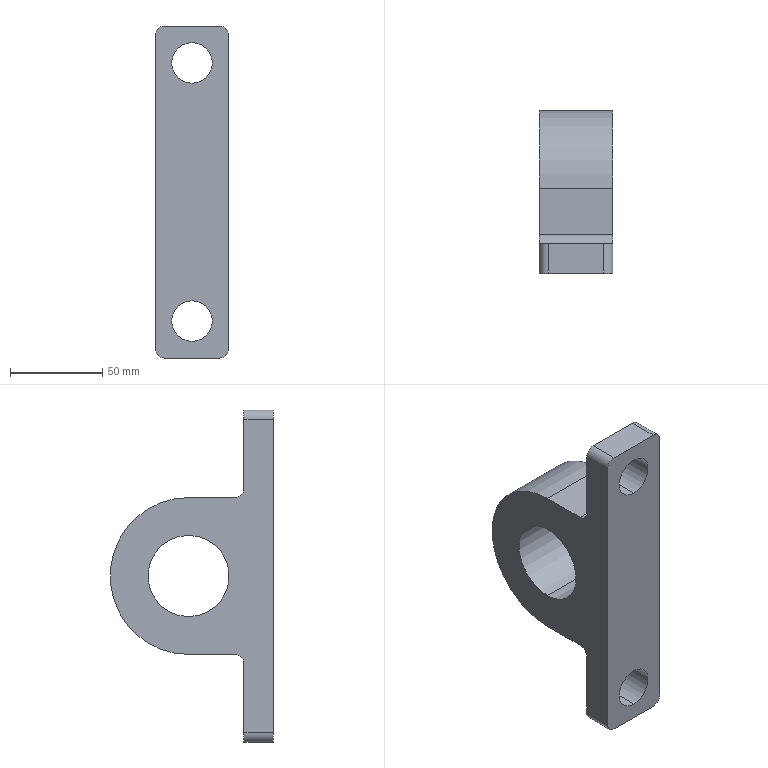Part | SolidWorks | features Extrusion 1, Fillet 1, ICE 1 | 1 solid | 22 faces | box 40 x 88.5 x 180 mm | volume 257790 mm3 | cylinder 13 | plane 9 | commonest cylinder face diameters 10 x6 22 x4 44 x2 85 x1
STEP:
#1=CARTESIAN_POINT('',(20.,46.,22.));
#2=VERTEX_POINT('',#1);
#3=CARTESIAN_POINT('',(20.,46.,-22.));
#4=VERTEX_POINT('',#3);
#5=CARTESIAN_POINT('',(20.,46.,0.));
#6=DIRECTION('',(1.,0.,0.));
#7=DIRECTION('',(0.,0.,-1.));
#8=AXIS2_PLACEMENT_3D('',#5,#6,#7);
#9=CIRCLE('',#8,22.);
#10=EDGE_CURVE('',#2,#4,#9,.T.);
#11=ORIENTED_EDGE('',*,*,#10,.T.);
#12=CARTESIAN_POINT('',(-20.,46.,-22.));
#13=VERTEX_POINT('',#12);
#14=CARTESIAN_POINT('',(20.,46.,-22.));
#15=DIRECTION('',(-1.,0.,0.));
#16=VECTOR('',#15,1000.);
#17=LINE('',#14,#16);
#18=EDGE_CURVE('',#4,#13,#17,.T.);
#19=ORIENTED_EDGE('',*,*,#18,.T.);
#20=CARTESIAN_POINT('',(-20.,46.,22.));
#21=VERTEX_POINT('',#20);
#22=CARTESIAN_POINT('',(-20.,46.,0.));
#23=DIRECTION('',(1.,0.,0.));
#24=DIRECTION('',(0.,0.,-1.));
#25=AXIS2_PLACEMENT_3D('',#22,#23,#24);
#26=CIRCLE('',#25,22.);
#27=EDGE_CURVE('',#21,#13,#26,.T.);
#28=ORIENTED_EDGE('',*,*,#27,.F.);
#29=CARTESIAN_POINT('',(20.,46.,22.));
#30=DIRECTION('',(-1.,0.,0.));
#31=VECTOR('',#30,1000.);
#32=LINE('',#29,#31);
#33=EDGE_CURVE('',#2,#21,#32,.T.);
#34=ORIENTED_EDGE('',*,*,#33,.F.);
#35=EDGE_LOOP('',(#11,#19,#28,#34));
#36=FACE_OUTER_BOUND('',#35,.T.);
#37=CARTESIAN_POINT('',(20.,46.,0.));
#38=DIRECTION('',(-1.,0.,0.));
#39=DIRECTION('',(0.,0.,1.));
#40=AXIS2_PLACEMENT_3D('',#37,#38,#39);
#41=CYLINDRICAL_SURFACE('',#40,22.);
#42=ADVANCED_FACE('',(#36),#41,.F.);
#43=CARTESIAN_POINT('',(0.,16.,59.));
#44=VERTEX_POINT('',#43);
#45=CARTESIAN_POINT('',(0.,16.,81.));
#46=VERTEX_POINT('',#45);
#47=CARTESIAN_POINT('',(0.,16.,70.));
#48=DIRECTION('',(0.,1.,0.));
#49=DIRECTION('',(0.,0.,-1.));
#50=AXIS2_PLACEMENT_3D('',#47,#48,#49);
#51=CIRCLE('',#50,11.);
#52=EDGE_CURVE('',#44,#46,#51,.T.);
#53=ORIENTED_EDGE('',*,*,#52,.T.);
#54=CARTESIAN_POINT('',(0.,0.,81.));
#55=VERTEX_POINT('',#54);
#56=CARTESIAN_POINT('',(0.,16.,81.));
#57=DIRECTION('',(0.,-1.,0.));
#58=VECTOR('',#57,1000.);
#59=LINE('',#56,#58);
#60=EDGE_CURVE('',#46,#55,#59,.T.);
#61=ORIENTED_EDGE('',*,*,#60,.T.);
#62=CARTESIAN_POINT('',(0.,0.,59.));
#63=VERTEX_POINT('',#62);
#64=CARTESIAN_POINT('',(0.,0.,70.));
#65=DIRECTION('',(0.,1.,0.));
#66=DIRECTION('',(0.,0.,-1.));
#67=AXIS2_PLACEMENT_3D('',#64,#65,#66);
#68=CIRCLE('',#67,11.);
#69=EDGE_CURVE('',#63,#55,#68,.T.);
#70=ORIENTED_EDGE('',*,*,#69,.F.);
#71=CARTESIAN_POINT('',(0.,16.,59.));
#72=DIRECTION('',(0.,-1.,0.));
#73=VECTOR('',#72,1000.);
#74=LINE('',#71,#73);
#75=EDGE_CURVE('',#44,#63,#74,.T.);
#76=ORIENTED_EDGE('',*,*,#75,.F.);
#77=EDGE_LOOP('',(#53,#61,#70,#76));
#78=FACE_OUTER_BOUND('',#77,.T.);
#79=CARTESIAN_POINT('',(0.,16.,70.));
#80=DIRECTION('',(0.,-1.,0.));
#81=DIRECTION('',(0.,0.,-1.));
#82=AXIS2_PLACEMENT_3D('',#79,#80,#81);
#83=CYLINDRICAL_SURFACE('',#82,11.);
#84=ADVANCED_FACE('',(#78),#83,.F.);
#85=CARTESIAN_POINT('',(0.,16.,-81.));
#86=VERTEX_POINT('',#85);
#87=CARTESIAN_POINT('',(0.,16.,-59.));
#88=VERTEX_POINT('',#87);
#89=CARTESIAN_POINT('',(0.,16.,-70.));
#90=DIRECTION('',(0.,1.,0.));
#91=DIRECTION('',(0.,0.,1.));
#92=AXIS2_PLACEMENT_3D('',#89,#90,#91);
#93=CIRCLE('',#92,11.);
#94=EDGE_CURVE('',#86,#88,#93,.T.);
#95=ORIENTED_EDGE('',*,*,#94,.T.);
#96=CARTESIAN_POINT('',(0.,0.,-59.));
#97=VERTEX_POINT('',#96);
#98=CARTESIAN_POINT('',(0.,16.,-59.));
#99=DIRECTION('',(0.,-1.,0.));
#100=VECTOR('',#99,1000.);
#101=LINE('',#98,#100);
#102=EDGE_CURVE('',#88,#97,#101,.T.);
#103=ORIENTED_EDGE('',*,*,#102,.T.);
#104=CARTESIAN_POINT('',(0.,0.,-81.));
#105=VERTEX_POINT('',#104);
#106=CARTESIAN_POINT('',(0.,0.,-70.));
#107=DIRECTION('',(0.,1.,0.));
#108=DIRECTION('',(0.,0.,1.));
#109=AXIS2_PLACEMENT_3D('',#106,#107,#108);
#110=CIRCLE('',#109,11.);
#111=EDGE_CURVE('',#105,#97,#110,.T.);
#112=ORIENTED_EDGE('',*,*,#111,.F.);
#113=CARTESIAN_POINT('',(0.,16.,-81.));
#114=DIRECTION('',(0.,-1.,0.));
#115=VECTOR('',#114,1000.);
#116=LINE('',#113,#115);
#117=EDGE_CURVE('',#86,#105,#116,.T.);
#118=ORIENTED_EDGE('',*,*,#117,.F.);
#119=EDGE_LOOP('',(#95,#103,#112,#118));
#120=FACE_OUTER_BOUND('',#119,.T.);
#121=CARTESIAN_POINT('',(0.,16.,-70.));
#122=DIRECTION('',(0.,-1.,0.));
#123=DIRECTION('',(0.,0.,-1.));
#124=AXIS2_PLACEMENT_3D('',#121,#122,#123);
#125=CYLINDRICAL_SURFACE('',#124,11.);
#126=ADVANCED_FACE('',(#120),#125,.F.);
#127=ORIENTED_EDGE('',*,*,#52,.F.);
#128=CARTESIAN_POINT('',(0.,16.,70.));
#129=DIRECTION('',(0.,1.,0.));
#130=DIRECTION('',(0.,0.,-1.));
#131=AXIS2_PLACEMENT_3D('',#128,#129,#130);
#132=CIRCLE('',#131,11.);
#133=EDGE_CURVE('',#46,#44,#132,.T.);
#134=ORIENTED_EDGE('',*,*,#133,.F.);
#135=EDGE_LOOP('',(#127,#134));
#136=FACE_BOUND('',#135,.T.);
#137=CARTESIAN_POINT('',(20.,16.,85.));
#138=VERTEX_POINT('',#137);
#139=CARTESIAN_POINT('',(20.,16.,47.5));
#140=VERTEX_POINT('',#139);
#141=CARTESIAN_POINT('',(20.,16.,-90.));
#142=DIRECTION('',(0.,0.,-1.));
#143=VECTOR('',#142,1000.);
#144=LINE('',#141,#143);
#145=EDGE_CURVE('',#138,#140,#144,.T.);
#146=ORIENTED_EDGE('',*,*,#145,.T.);
#147=CARTESIAN_POINT('',(-20.,16.,47.5));
#148=VERTEX_POINT('',#147);
#149=CARTESIAN_POINT('',(-20.,16.,47.5));
#150=DIRECTION('',(-1.,0.,0.));
#151=VECTOR('',#150,1000.);
#152=LINE('',#149,#151);
#153=EDGE_CURVE('',#140,#148,#152,.T.);
#154=ORIENTED_EDGE('',*,*,#153,.T.);
#155=CARTESIAN_POINT('',(-20.,16.,85.));
#156=VERTEX_POINT('',#155);
#157=CARTESIAN_POINT('',(-20.,16.,-90.));
#158=DIRECTION('',(0.,0.,1.));
#159=VECTOR('',#158,1000.);
#160=LINE('',#157,#159);
#161=EDGE_CURVE('',#148,#156,#160,.T.);
#162=ORIENTED_EDGE('',*,*,#161,.T.);
#163=CARTESIAN_POINT('',(-15.,16.,90.));
#164=VERTEX_POINT('',#163);
#165=CARTESIAN_POINT('',(-15.,16.,85.));
#166=DIRECTION('',(0.,1.,0.));
#167=DIRECTION('',(0.,0.,1.));
#168=AXIS2_PLACEMENT_3D('',#165,#166,#167);
#169=CIRCLE('',#168,5.);
#170=EDGE_CURVE('',#156,#164,#169,.T.);
#171=ORIENTED_EDGE('',*,*,#170,.T.);
#172=CARTESIAN_POINT('',(15.,16.,90.));
#173=VERTEX_POINT('',#172);
#174=CARTESIAN_POINT('',(-20.,16.,90.));
#175=DIRECTION('',(1.,0.,0.));
#176=VECTOR('',#175,1000.);
#177=LINE('',#174,#176);
#178=EDGE_CURVE('',#164,#173,#177,.T.);
#179=ORIENTED_EDGE('',*,*,#178,.T.);
#180=CARTESIAN_POINT('',(15.,16.,85.));
#181=DIRECTION('',(0.,1.,0.));
#182=DIRECTION('',(0.,0.,1.));
#183=AXIS2_PLACEMENT_3D('',#180,#181,#182);
#184=CIRCLE('',#183,5.);
#185=EDGE_CURVE('',#173,#138,#184,.T.);
#186=ORIENTED_EDGE('',*,*,#185,.T.);
#187=EDGE_LOOP('',(#146,#154,#162,#171,#179,#186));
#188=FACE_OUTER_BOUND('',#187,.T.);
#189=CARTESIAN_POINT('',(-20.,16.,90.));
#190=DIRECTION('',(0.,1.,0.));
#191=DIRECTION('',(0.,0.,1.));
#192=AXIS2_PLACEMENT_3D('',#189,#190,#191);
#193=PLANE('',#192);
#194=ADVANCED_FACE('',(#136,#188),#193,.T.);
#195=CARTESIAN_POINT('',(20.,16.,-47.5));
#196=VERTEX_POINT('',#195);
#197=CARTESIAN_POINT('',(20.,16.,-85.));
#198=VERTEX_POINT('',#197);
#199=CARTESIAN_POINT('',(20.,16.,-90.));
#200=DIRECTION('',(0.,0.,-1.));
#201=VECTOR('',#200,1000.);
#202=LINE('',#199,#201);
#203=EDGE_CURVE('',#196,#198,#202,.T.);
#204=ORIENTED_EDGE('',*,*,#203,.T.);
#205=CARTESIAN_POINT('',(15.,16.,-90.));
#206=VERTEX_POINT('',#205);
#207=CARTESIAN_POINT('',(15.,16.,-85.));
#208=DIRECTION('',(0.,1.,0.));
#209=DIRECTION('',(0.,0.,1.));
#210=AXIS2_PLACEMENT_3D('',#207,#208,#209);
#211=CIRCLE('',#210,5.);
#212=EDGE_CURVE('',#198,#206,#211,.T.);
#213=ORIENTED_EDGE('',*,*,#212,.T.);
#214=CARTESIAN_POINT('',(-15.,16.,-90.));
#215=VERTEX_POINT('',#214);
#216=CARTESIAN_POINT('',(-20.,16.,-90.));
#217=DIRECTION('',(-1.,0.,0.));
#218=VECTOR('',#217,1000.);
#219=LINE('',#216,#218);
#220=EDGE_CURVE('',#206,#215,#219,.T.);
#221=ORIENTED_EDGE('',*,*,#220,.T.);
#222=CARTESIAN_POINT('',(-20.,16.,-85.));
#223=VERTEX_POINT('',#222);
#224=CARTESIAN_POINT('',(-15.,16.,-85.));
#225=DIRECTION('',(0.,1.,0.));
#226=DIRECTION('',(0.,0.,1.));
#227=AXIS2_PLACEMENT_3D('',#224,#225,#226);
#228=CIRCLE('',#227,5.);
#229=EDGE_CURVE('',#215,#223,#228,.T.);
#230=ORIENTED_EDGE('',*,*,#229,.T.);
#231=CARTESIAN_POINT('',(-20.,16.,-47.5));
#232=VERTEX_POINT('',#231);
#233=CARTESIAN_POINT('',(-20.,16.,-90.));
#234=DIRECTION('',(0.,0.,1.));
#235=VECTOR('',#234,1000.);
#236=LINE('',#233,#235);
#237=EDGE_CURVE('',#223,#232,#236,.T.);
#238=ORIENTED_EDGE('',*,*,#237,.T.);
#239=CARTESIAN_POINT('',(-20.,16.,-47.5));
#240=DIRECTION('',(1.,0.,0.));
#241=VECTOR('',#240,1000.);
#242=LINE('',#239,#241);
#243=EDGE_CURVE('',#232,#196,#242,.T.);
#244=ORIENTED_EDGE('',*,*,#243,.T.);
#245=EDGE_LOOP('',(#204,#213,#221,#230,#238,#244));
#246=FACE_OUTER_BOUND('',#245,.T.);
#247=ORIENTED_EDGE('',*,*,#94,.F.);
#248=CARTESIAN_POINT('',(0.,16.,-70.));
#249=DIRECTION('',(0.,1.,0.));
#250=DIRECTION('',(0.,0.,1.));
#251=AXIS2_PLACEMENT_3D('',#248,#249,#250);
#252=CIRCLE('',#251,11.);
#253=EDGE_CURVE('',#88,#86,#252,.T.);
#254=ORIENTED_EDGE('',*,*,#253,.F.);
#255=EDGE_LOOP('',(#247,#254));
#256=FACE_BOUND('',#255,.T.);
#257=CARTESIAN_POINT('',(-20.,16.,90.));
#258=DIRECTION('',(0.,1.,0.));
#259=DIRECTION('',(0.,0.,1.));
#260=AXIS2_PLACEMENT_3D('',#257,#258,#259);
#261=PLANE('',#260);
#262=ADVANCED_FACE('',(#246,#256),#261,.T.);
#263=ORIENTED_EDGE('',*,*,#111,.T.);
#264=CARTESIAN_POINT('',(0.,0.,-70.));
#265=DIRECTION('',(0.,1.,0.));
#266=DIRECTION('',(0.,0.,1.));
#267=AXIS2_PLACEMENT_3D('',#264,#265,#266);
#268=CIRCLE('',#267,11.);
#269=EDGE_CURVE('',#97,#105,#268,.T.);
#270=ORIENTED_EDGE('',*,*,#269,.T.);
#271=EDGE_LOOP('',(#263,#270));
#272=FACE_BOUND('',#271,.T.);
#273=CARTESIAN_POINT('',(20.,0.,85.));
#274=VERTEX_POINT('',#273);
#275=CARTESIAN_POINT('',(20.,0.,-85.));
#276=VERTEX_POINT('',#275);
#277=CARTESIAN_POINT('',(20.,0.,-90.));
#278=DIRECTION('',(0.,0.,-1.));
#279=VECTOR('',#278,1000.);
#280=LINE('',#277,#279);
#281=EDGE_CURVE('',#274,#276,#280,.T.);
#282=ORIENTED_EDGE('',*,*,#281,.F.);
#283=CARTESIAN_POINT('',(15.,0.,90.));
#284=VERTEX_POINT('',#283);
#285=CARTESIAN_POINT('',(15.,0.,85.));
#286=DIRECTION('',(0.,-1.,0.));
#287=DIRECTION('',(0.,0.,1.));
#288=AXIS2_PLACEMENT_3D('',#285,#286,#287);
#289=CIRCLE('',#288,5.);
#290=EDGE_CURVE('',#274,#284,#289,.T.);
#291=ORIENTED_EDGE('',*,*,#290,.T.);
#292=CARTESIAN_POINT('',(-15.,0.,90.));
#293=VERTEX_POINT('',#292);
#294=CARTESIAN_POINT('',(-20.,0.,90.));
#295=DIRECTION('',(1.,0.,0.));
#296=VECTOR('',#295,1000.);
#297=LINE('',#294,#296);
#298=EDGE_CURVE('',#293,#284,#297,.T.);
#299=ORIENTED_EDGE('',*,*,#298,.F.);
#300=CARTESIAN_POINT('',(-20.,0.,85.));
#301=VERTEX_POINT('',#300);
#302=CARTESIAN_POINT('',(-15.,0.,85.));
#303=DIRECTION('',(0.,-1.,0.));
#304=DIRECTION('',(0.,0.,1.));
#305=AXIS2_PLACEMENT_3D('',#302,#303,#304);
#306=CIRCLE('',#305,5.);
#307=EDGE_CURVE('',#293,#301,#306,.T.);
#308=ORIENTED_EDGE('',*,*,#307,.T.);
#309=CARTESIAN_POINT('',(-20.,0.,-85.));
#310=VERTEX_POINT('',#309);
#311=CARTESIAN_POINT('',(-20.,0.,-90.));
#312=DIRECTION('',(0.,0.,1.));
#313=VECTOR('',#312,1000.);
#314=LINE('',#311,#313);
#315=EDGE_CURVE('',#310,#301,#314,.T.);
#316=ORIENTED_EDGE('',*,*,#315,.F.);
#317=CARTESIAN_POINT('',(-15.,0.,-90.));
#318=VERTEX_POINT('',#317);
#319=CARTESIAN_POINT('',(-15.,0.,-85.));
#320=DIRECTION('',(0.,-1.,0.));
#321=DIRECTION('',(0.,0.,1.));
#322=AXIS2_PLACEMENT_3D('',#319,#320,#321);
#323=CIRCLE('',#322,5.);
#324=EDGE_CURVE('',#310,#318,#323,.T.);
#325=ORIENTED_EDGE('',*,*,#324,.T.);
#326=CARTESIAN_POINT('',(15.,0.,-90.));
#327=VERTEX_POINT('',#326);
#328=CARTESIAN_POINT('',(-20.,0.,-90.));
#329=DIRECTION('',(-1.,0.,0.));
#330=VECTOR('',#329,1000.);
#331=LINE('',#328,#330);
#332=EDGE_CURVE('',#327,#318,#331,.T.);
#333=ORIENTED_EDGE('',*,*,#332,.F.);
#334=CARTESIAN_POINT('',(15.,0.,-85.));
#335=DIRECTION('',(0.,-1.,0.));
#336=DIRECTION('',(0.,0.,1.));
#337=AXIS2_PLACEMENT_3D('',#334,#335,#336);
#338=CIRCLE('',#337,5.);
#339=EDGE_CURVE('',#327,#276,#338,.T.);
#340=ORIENTED_EDGE('',*,*,#339,.T.);
#341=EDGE_LOOP('',(#282,#291,#299,#308,#316,#325,#333,#340));
#342=FACE_OUTER_BOUND('',#341,.T.);
#343=ORIENTED_EDGE('',*,*,#69,.T.);
#344=CARTESIAN_POINT('',(0.,0.,70.));
#345=DIRECTION('',(0.,1.,0.));
#346=DIRECTION('',(0.,0.,-1.));
#347=AXIS2_PLACEMENT_3D('',#344,#345,#346);
#348=CIRCLE('',#347,11.);
#349=EDGE_CURVE('',#55,#63,#348,.T.);
#350=ORIENTED_EDGE('',*,*,#349,.T.);
#351=EDGE_LOOP('',(#343,#350));
#352=FACE_BOUND('',#351,.T.);
#353=CARTESIAN_POINT('',(-20.,0.,90.));
#354=DIRECTION('',(0.,1.,0.));
#355=DIRECTION('',(0.,0.,1.));
#356=AXIS2_PLACEMENT_3D('',#353,#354,#355);
#357=PLANE('',#356);
#358=ADVANCED_FACE('',(#272,#342,#352),#357,.F.);
#359=ORIENTED_EDGE('',*,*,#315,.T.);
#360=CARTESIAN_POINT('',(-20.,16.,85.));
#361=DIRECTION('',(0.,1.,0.));
#362=VECTOR('',#361,1000.);
#363=LINE('',#360,#362);
#364=EDGE_CURVE('',#301,#156,#363,.T.);
#365=ORIENTED_EDGE('',*,*,#364,.T.);
#366=ORIENTED_EDGE('',*,*,#161,.F.);
#367=CARTESIAN_POINT('',(-20.,21.,42.5));
#368=VERTEX_POINT('',#367);
#369=CARTESIAN_POINT('',(-20.,21.,47.5));
#370=DIRECTION('',(1.,0.,0.));
#371=DIRECTION('',(0.,0.,-1.));
#372=AXIS2_PLACEMENT_3D('',#369,#370,#371);
#373=CIRCLE('',#372,5.);
#374=EDGE_CURVE('',#148,#368,#373,.T.);
#375=ORIENTED_EDGE('',*,*,#374,.T.);
#376=CARTESIAN_POINT('',(-20.,46.,42.5));
#377=VERTEX_POINT('',#376);
#378=CARTESIAN_POINT('',(-20.,46.,42.5));
#379=DIRECTION('',(0.,-1.,0.));
#380=VECTOR('',#379,1000.);
#381=LINE('',#378,#380);
#382=EDGE_CURVE('',#377,#368,#381,.T.);
#383=ORIENTED_EDGE('',*,*,#382,.F.);
#384=CARTESIAN_POINT('',(-20.,46.,-42.5));
#385=VERTEX_POINT('',#384);
#386=CARTESIAN_POINT('',(-20.,46.,0.));
#387=DIRECTION('',(1.,0.,0.));
#388=DIRECTION('',(0.,0.,-1.));
#389=AXIS2_PLACEMENT_3D('',#386,#387,#388);
#390=CIRCLE('',#389,42.5);
#391=EDGE_CURVE('',#385,#377,#390,.T.);
#392=ORIENTED_EDGE('',*,*,#391,.F.);
#393=CARTESIAN_POINT('',(-20.,21.,-42.5));
#394=VERTEX_POINT('',#393);
#395=CARTESIAN_POINT('',(-20.,46.,-42.5));
#396=DIRECTION('',(0.,1.,0.));
#397=VECTOR('',#396,1000.);
#398=LINE('',#395,#397);
#399=EDGE_CURVE('',#394,#385,#398,.T.);
#400=ORIENTED_EDGE('',*,*,#399,.F.);
#401=CARTESIAN_POINT('',(-20.,21.,-47.5));
#402=DIRECTION('',(1.,0.,0.));
#403=DIRECTION('',(0.,0.,-1.));
#404=AXIS2_PLACEMENT_3D('',#401,#402,#403);
#405=CIRCLE('',#404,5.);
#406=EDGE_CURVE('',#394,#232,#405,.T.);
#407=ORIENTED_EDGE('',*,*,#406,.T.);
#408=ORIENTED_EDGE('',*,*,#237,.F.);
#409=CARTESIAN_POINT('',(-20.,16.,-85.));
#410=DIRECTION('',(0.,-1.,0.));
#411=VECTOR('',#410,1000.);
#412=LINE('',#409,#411);
#413=EDGE_CURVE('',#223,#310,#412,.T.);
#414=ORIENTED_EDGE('',*,*,#413,.T.);
#415=EDGE_LOOP('',(#359,#365,#366,#375,#383,#392,#400,#407,#408,#414));
#416=FACE_OUTER_BOUND('',#415,.T.);
#417=ORIENTED_EDGE('',*,*,#27,.T.);
#418=CARTESIAN_POINT('',(-20.,46.,0.));
#419=DIRECTION('',(1.,0.,0.));
#420=DIRECTION('',(0.,0.,-1.));
#421=AXIS2_PLACEMENT_3D('',#418,#419,#420);
#422=CIRCLE('',#421,22.);
#423=EDGE_CURVE('',#13,#21,#422,.T.);
#424=ORIENTED_EDGE('',*,*,#423,.T.);
#425=EDGE_LOOP('',(#417,#424));
#426=FACE_BOUND('',#425,.T.);
#427=CARTESIAN_POINT('',(-20.,16.,-90.));
#428=DIRECTION('',(1.,0.,0.));
#429=DIRECTION('',(0.,0.,-1.));
#430=AXIS2_PLACEMENT_3D('',#427,#428,#429);
#431=PLANE('',#430);
#432=ADVANCED_FACE('',(#416,#426),#431,.F.);
#433=ORIENTED_EDGE('',*,*,#298,.T.);
#434=CARTESIAN_POINT('',(15.,16.,90.));
#435=DIRECTION('',(0.,1.,0.));
#436=VECTOR('',#435,1000.);
#437=LINE('',#434,#436);
#438=EDGE_CURVE('',#284,#173,#437,.T.);
#439=ORIENTED_EDGE('',*,*,#438,.T.);
#440=ORIENTED_EDGE('',*,*,#178,.F.);
#441=CARTESIAN_POINT('',(-15.,16.,90.));
#442=DIRECTION('',(0.,-1.,0.));
#443=VECTOR('',#442,1000.);
#444=LINE('',#441,#443);
#445=EDGE_CURVE('',#164,#293,#444,.T.);
#446=ORIENTED_EDGE('',*,*,#445,.T.);
#447=EDGE_LOOP('',(#433,#439,#440,#446));
#448=FACE_OUTER_BOUND('',#447,.T.);
#449=CARTESIAN_POINT('',(-20.,16.,90.));
#450=DIRECTION('',(0.,0.,-1.));
#451=DIRECTION('',(-1.,0.,0.));
#452=AXIS2_PLACEMENT_3D('',#449,#450,#451);
#453=PLANE('',#452);
#454=ADVANCED_FACE('',(#448),#453,.F.);
#455=ORIENTED_EDGE('',*,*,#145,.F.);
#456=CARTESIAN_POINT('',(20.,16.,85.));
#457=DIRECTION('',(0.,-1.,0.));
#458=VECTOR('',#457,1000.);
#459=LINE('',#456,#458);
#460=EDGE_CURVE('',#138,#274,#459,.T.);
#461=ORIENTED_EDGE('',*,*,#460,.T.);
#462=ORIENTED_EDGE('',*,*,#281,.T.);
#463=CARTESIAN_POINT('',(20.,16.,-85.));
#464=DIRECTION('',(0.,1.,0.));
#465=VECTOR('',#464,1000.);
#466=LINE('',#463,#465);
#467=EDGE_CURVE('',#276,#198,#466,.T.);
#468=ORIENTED_EDGE('',*,*,#467,.T.);
#469=ORIENTED_EDGE('',*,*,#203,.F.);
#470=CARTESIAN_POINT('',(20.,21.,-42.5));
#471=VERTEX_POINT('',#470);
#472=CARTESIAN_POINT('',(20.,21.,-47.5));
#473=DIRECTION('',(-1.,0.,0.));
#474=DIRECTION('',(0.,0.,1.));
#475=AXIS2_PLACEMENT_3D('',#472,#473,#474);
#476=CIRCLE('',#475,5.);
#477=EDGE_CURVE('',#196,#471,#476,.T.);
#478=ORIENTED_EDGE('',*,*,#477,.T.);
#479=CARTESIAN_POINT('',(20.,46.,-42.5));
#480=VERTEX_POINT('',#479);
#481=CARTESIAN_POINT('',(20.,46.,-42.5));
#482=DIRECTION('',(0.,1.,0.));
#483=VECTOR('',#482,1000.);
#484=LINE('',#481,#483);
#485=EDGE_CURVE('',#471,#480,#484,.T.);
#486=ORIENTED_EDGE('',*,*,#485,.T.);
#487=CARTESIAN_POINT('',(20.,46.,42.5));
#488=VERTEX_POINT('',#487);
#489=CARTESIAN_POINT('',(20.,46.,0.));
#490=DIRECTION('',(1.,0.,0.));
#491=DIRECTION('',(0.,0.,-1.));
#492=AXIS2_PLACEMENT_3D('',#489,#490,#491);
#493=CIRCLE('',#492,42.5);
#494=EDGE_CURVE('',#480,#488,#493,.T.);
#495=ORIENTED_EDGE('',*,*,#494,.T.);
#496=CARTESIAN_POINT('',(20.,21.,42.5));
#497=VERTEX_POINT('',#496);
#498=CARTESIAN_POINT('',(20.,46.,42.5));
#499=DIRECTION('',(0.,-1.,0.));
#500=VECTOR('',#499,1000.);
#501=LINE('',#498,#500);
#502=EDGE_CURVE('',#488,#497,#501,.T.);
#503=ORIENTED_EDGE('',*,*,#502,.T.);
#504=CARTESIAN_POINT('',(20.,21.,47.5));
#505=DIRECTION('',(-1.,0.,0.));
#506=DIRECTION('',(0.,0.,1.));
#507=AXIS2_PLACEMENT_3D('',#504,#505,#506);
#508=CIRCLE('',#507,5.);
#509=EDGE_CURVE('',#497,#140,#508,.T.);
#510=ORIENTED_EDGE('',*,*,#509,.T.);
#511=EDGE_LOOP('',(#455,#461,#462,#468,#469,#478,#486,#495,#503,#510));
#512=FACE_OUTER_BOUND('',#511,.T.);
#513=ORIENTED_EDGE('',*,*,#10,.F.);
#514=CARTESIAN_POINT('',(20.,46.,0.));
#515=DIRECTION('',(1.,0.,0.));
#516=DIRECTION('',(0.,0.,-1.));
#517=AXIS2_PLACEMENT_3D('',#514,#515,#516);
#518=CIRCLE('',#517,22.);
#519=EDGE_CURVE('',#4,#2,#518,.T.);
#520=ORIENTED_EDGE('',*,*,#519,.F.);
#521=EDGE_LOOP('',(#513,#520));
#522=FACE_BOUND('',#521,.T.);
#523=CARTESIAN_POINT('',(20.,16.,-90.));
#524=DIRECTION('',(-1.,0.,0.));
#525=DIRECTION('',(0.,0.,1.));
#526=AXIS2_PLACEMENT_3D('',#523,#524,#525);
#527=PLANE('',#526);
#528=ADVANCED_FACE('',(#512,#522),#527,.F.);
#529=ORIENTED_EDGE('',*,*,#220,.F.);
#530=CARTESIAN_POINT('',(15.,16.,-90.));
#531=DIRECTION('',(0.,-1.,0.));
#532=VECTOR('',#531,1000.);
#533=LINE('',#530,#532);
#534=EDGE_CURVE('',#206,#327,#533,.T.);
#535=ORIENTED_EDGE('',*,*,#534,.T.);
#536=ORIENTED_EDGE('',*,*,#332,.T.);
#537=CARTESIAN_POINT('',(-15.,16.,-90.));
#538=DIRECTION('',(0.,1.,0.));
#539=VECTOR('',#538,1000.);
#540=LINE('',#537,#539);
#541=EDGE_CURVE('',#318,#215,#540,.T.);
#542=ORIENTED_EDGE('',*,*,#541,.T.);
#543=EDGE_LOOP('',(#529,#535,#536,#542));
#544=FACE_OUTER_BOUND('',#543,.T.);
#545=CARTESIAN_POINT('',(-20.,16.,-90.));
#546=DIRECTION('',(0.,0.,1.));
#547=DIRECTION('',(1.,0.,0.));
#548=AXIS2_PLACEMENT_3D('',#545,#546,#547);
#549=PLANE('',#548);
#550=ADVANCED_FACE('',(#544),#549,.F.);
#551=ORIENTED_EDGE('',*,*,#102,.F.);
#552=ORIENTED_EDGE('',*,*,#253,.T.);
#553=ORIENTED_EDGE('',*,*,#117,.T.);
#554=ORIENTED_EDGE('',*,*,#269,.F.);
#555=EDGE_LOOP('',(#551,#552,#553,#554));
#556=FACE_OUTER_BOUND('',#555,.T.);
#557=CARTESIAN_POINT('',(0.,16.,-70.));
#558=DIRECTION('',(0.,-1.,0.));
#559=DIRECTION('',(0.,0.,-1.));
#560=AXIS2_PLACEMENT_3D('',#557,#558,#559);
#561=CYLINDRICAL_SURFACE('',#560,11.);
#562=ADVANCED_FACE('',(#556),#561,.F.);
#563=ORIENTED_EDGE('',*,*,#60,.F.);
#564=ORIENTED_EDGE('',*,*,#133,.T.);
#565=ORIENTED_EDGE('',*,*,#75,.T.);
#566=ORIENTED_EDGE('',*,*,#349,.F.);
#567=EDGE_LOOP('',(#563,#564,#565,#566));
#568=FACE_OUTER_BOUND('',#567,.T.);
#569=CARTESIAN_POINT('',(0.,16.,70.));
#570=DIRECTION('',(0.,-1.,0.));
#571=DIRECTION('',(0.,0.,-1.));
#572=AXIS2_PLACEMENT_3D('',#569,#570,#571);
#573=CYLINDRICAL_SURFACE('',#572,11.);
#574=ADVANCED_FACE('',(#568),#573,.F.);
#575=ORIENTED_EDGE('',*,*,#391,.T.);
#576=CARTESIAN_POINT('',(20.,46.,42.5));
#577=DIRECTION('',(-1.,0.,0.));
#578=VECTOR('',#577,1000.);
#579=LINE('',#576,#578);
#580=EDGE_CURVE('',#488,#377,#579,.T.);
#581=ORIENTED_EDGE('',*,*,#580,.F.);
#582=ORIENTED_EDGE('',*,*,#494,.F.);
#583=CARTESIAN_POINT('',(20.,46.,-42.5));
#584=DIRECTION('',(-1.,0.,0.));
#585=VECTOR('',#584,1000.);
#586=LINE('',#583,#585);
#587=EDGE_CURVE('',#480,#385,#586,.T.);
#588=ORIENTED_EDGE('',*,*,#587,.T.);
#589=EDGE_LOOP('',(#575,#581,#582,#588));
#590=FACE_OUTER_BOUND('',#589,.T.);
#591=CARTESIAN_POINT('',(20.,46.,0.));
#592=DIRECTION('',(-1.,0.,0.));
#593=DIRECTION('',(0.,0.,1.));
#594=AXIS2_PLACEMENT_3D('',#591,#592,#593);
#595=CYLINDRICAL_SURFACE('',#594,42.5);
#596=ADVANCED_FACE('',(#590),#595,.T.);
#597=ORIENTED_EDGE('',*,*,#382,.T.);
#598=CARTESIAN_POINT('',(20.,21.,42.5));
#599=DIRECTION('',(1.,0.,0.));
#600=VECTOR('',#599,1000.);
#601=LINE('',#598,#600);
#602=EDGE_CURVE('',#368,#497,#601,.T.);
#603=ORIENTED_EDGE('',*,*,#602,.T.);
#604=ORIENTED_EDGE('',*,*,#502,.F.);
#605=ORIENTED_EDGE('',*,*,#580,.T.);
#606=EDGE_LOOP('',(#597,#603,#604,#605));
#607=FACE_OUTER_BOUND('',#606,.T.);
#608=CARTESIAN_POINT('',(20.,46.,42.5));
#609=DIRECTION('',(0.,0.,-1.));
#610=DIRECTION('',(0.,1.,0.));
#611=AXIS2_PLACEMENT_3D('',#608,#609,#610);
#612=PLANE('',#611);
#613=ADVANCED_FACE('',(#607),#612,.F.);
#614=ORIENTED_EDGE('',*,*,#485,.F.);
#615=CARTESIAN_POINT('',(20.,21.,-42.5));
#616=DIRECTION('',(-1.,0.,0.));
#617=VECTOR('',#616,1000.);
#618=LINE('',#615,#617);
#619=EDGE_CURVE('',#471,#394,#618,.T.);
#620=ORIENTED_EDGE('',*,*,#619,.T.);
#621=ORIENTED_EDGE('',*,*,#399,.T.);
#622=ORIENTED_EDGE('',*,*,#587,.F.);
#623=EDGE_LOOP('',(#614,#620,#621,#622));
#624=FACE_OUTER_BOUND('',#623,.T.);
#625=CARTESIAN_POINT('',(20.,46.,-42.5));
#626=DIRECTION('',(0.,0.,1.));
#627=DIRECTION('',(0.,-1.,0.));
#628=AXIS2_PLACEMENT_3D('',#625,#626,#627);
#629=PLANE('',#628);
#630=ADVANCED_FACE('',(#624),#629,.F.);
#631=ORIENTED_EDGE('',*,*,#18,.F.);
#632=ORIENTED_EDGE('',*,*,#519,.T.);
#633=ORIENTED_EDGE('',*,*,#33,.T.);
#634=ORIENTED_EDGE('',*,*,#423,.F.);
#635=EDGE_LOOP('',(#631,#632,#633,#634));
#636=FACE_OUTER_BOUND('',#635,.T.);
#637=CARTESIAN_POINT('',(20.,46.,0.));
#638=DIRECTION('',(-1.,0.,0.));
#639=DIRECTION('',(0.,0.,1.));
#640=AXIS2_PLACEMENT_3D('',#637,#638,#639);
#641=CYLINDRICAL_SURFACE('',#640,22.);
#642=ADVANCED_FACE('',(#636),#641,.F.);
#643=ORIENTED_EDGE('',*,*,#509,.F.);
#644=ORIENTED_EDGE('',*,*,#602,.F.);
#645=ORIENTED_EDGE('',*,*,#374,.F.);
#646=ORIENTED_EDGE('',*,*,#153,.F.);
#647=EDGE_LOOP('',(#643,#644,#645,#646));
#648=FACE_OUTER_BOUND('',#647,.T.);
#649=CARTESIAN_POINT('',(-20.,21.,47.5));
#650=DIRECTION('',(-1.,0.,0.));
#651=DIRECTION('',(0.,0.,1.));
#652=AXIS2_PLACEMENT_3D('',#649,#650,#651);
#653=CYLINDRICAL_SURFACE('',#652,5.);
#654=ADVANCED_FACE('',(#648),#653,.F.);
#655=ORIENTED_EDGE('',*,*,#185,.F.);
#656=ORIENTED_EDGE('',*,*,#438,.F.);
#657=ORIENTED_EDGE('',*,*,#290,.F.);
#658=ORIENTED_EDGE('',*,*,#460,.F.);
#659=EDGE_LOOP('',(#655,#656,#657,#658));
#660=FACE_OUTER_BOUND('',#659,.T.);
#661=CARTESIAN_POINT('',(15.,16.,85.));
#662=DIRECTION('',(0.,-1.,0.));
#663=DIRECTION('',(0.,0.,-1.));
#664=AXIS2_PLACEMENT_3D('',#661,#662,#663);
#665=CYLINDRICAL_SURFACE('',#664,5.);
#666=ADVANCED_FACE('',(#660),#665,.T.);
#667=ORIENTED_EDGE('',*,*,#170,.F.);
#668=ORIENTED_EDGE('',*,*,#364,.F.);
#669=ORIENTED_EDGE('',*,*,#307,.F.);
#670=ORIENTED_EDGE('',*,*,#445,.F.);
#671=EDGE_LOOP('',(#667,#668,#669,#670));
#672=FACE_OUTER_BOUND('',#671,.T.);
#673=CARTESIAN_POINT('',(-15.,16.,85.));
#674=DIRECTION('',(0.,-1.,0.));
#675=DIRECTION('',(0.,0.,-1.));
#676=AXIS2_PLACEMENT_3D('',#673,#674,#675);
#677=CYLINDRICAL_SURFACE('',#676,5.);
#678=ADVANCED_FACE('',(#672),#677,.T.);
#679=ORIENTED_EDGE('',*,*,#212,.F.);
#680=ORIENTED_EDGE('',*,*,#467,.F.);
#681=ORIENTED_EDGE('',*,*,#339,.F.);
#682=ORIENTED_EDGE('',*,*,#534,.F.);
#683=EDGE_LOOP('',(#679,#680,#681,#682));
#684=FACE_OUTER_BOUND('',#683,.T.);
#685=CARTESIAN_POINT('',(15.,16.,-85.));
#686=DIRECTION('',(0.,-1.,0.));
#687=DIRECTION('',(0.,0.,-1.));
#688=AXIS2_PLACEMENT_3D('',#685,#686,#687);
#689=CYLINDRICAL_SURFACE('',#688,5.);
#690=ADVANCED_FACE('',(#684),#689,.T.);
#691=ORIENTED_EDGE('',*,*,#229,.F.);
#692=ORIENTED_EDGE('',*,*,#541,.F.);
#693=ORIENTED_EDGE('',*,*,#324,.F.);
#694=ORIENTED_EDGE('',*,*,#413,.F.);
#695=EDGE_LOOP('',(#691,#692,#693,#694));
#696=FACE_OUTER_BOUND('',#695,.T.);
#697=CARTESIAN_POINT('',(-15.,16.,-85.));
#698=DIRECTION('',(0.,-1.,0.));
#699=DIRECTION('',(0.,0.,-1.));
#700=AXIS2_PLACEMENT_3D('',#697,#698,#699);
#701=CYLINDRICAL_SURFACE('',#700,5.);
#702=ADVANCED_FACE('',(#696),#701,.T.);
#703=ORIENTED_EDGE('',*,*,#477,.F.);
#704=ORIENTED_EDGE('',*,*,#243,.F.);
#705=ORIENTED_EDGE('',*,*,#406,.F.);
#706=ORIENTED_EDGE('',*,*,#619,.F.);
#707=EDGE_LOOP('',(#703,#704,#705,#706));
#708=FACE_OUTER_BOUND('',#707,.T.);
#709=CARTESIAN_POINT('',(20.,21.,-47.5));
#710=DIRECTION('',(-1.,0.,0.));
#711=DIRECTION('',(0.,0.,1.));
#712=AXIS2_PLACEMENT_3D('',#709,#710,#711);
#713=CYLINDRICAL_SURFACE('',#712,5.);
#714=ADVANCED_FACE('',(#708),#713,.F.);
#715=CLOSED_SHELL('',(#42,#84,#126,#194,#262,#358,#432,#454,#528,#550,#562,#574,#596,#613,#630,#642,#654,#666,#678,#690,#702,#714));
#716=MANIFOLD_SOLID_BREP('',#715);
#717=CARTESIAN_POINT('',(0.,0.,0.));
#718=DIRECTION('',(0.,0.,1.));
#719=DIRECTION('',(1.,0.,0.));
#720=AXIS2_PLACEMENT_3D('',#717,#718,#719);
#721=(LENGTH_UNIT()NAMED_UNIT(*)SI_UNIT(.MILLI.,.METRE.));
#722=UNCERTAINTY_MEASURE_WITH_UNIT(LENGTH_MEASURE(0.00001),#721,'','');
#723=(NAMED_UNIT(*)PLANE_ANGLE_UNIT()SI_UNIT($,.RADIAN.));
#724=(NAMED_UNIT(*)SI_UNIT($,.STERADIAN.)SOLID_ANGLE_UNIT());
#725=(GEOMETRIC_REPRESENTATION_CONTEXT(3)GLOBAL_UNCERTAINTY_ASSIGNED_CONTEXT((#722))GLOBAL_UNIT_ASSIGNED_CONTEXT((#721,#723,#724))REPRESENTATION_CONTEXT('',''));
#726=ADVANCED_BREP_SHAPE_REPRESENTATION('',(#716,#720),#725);